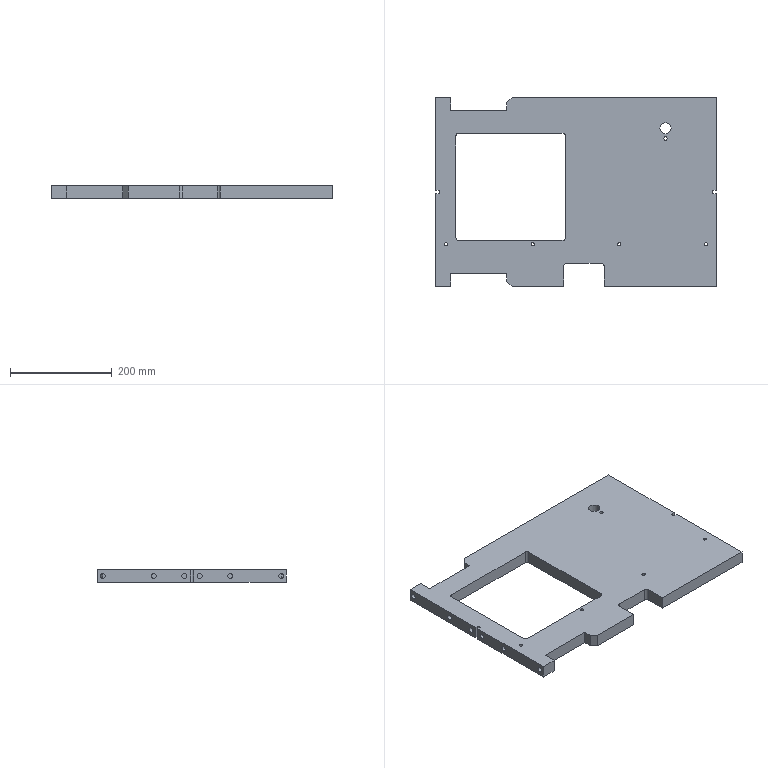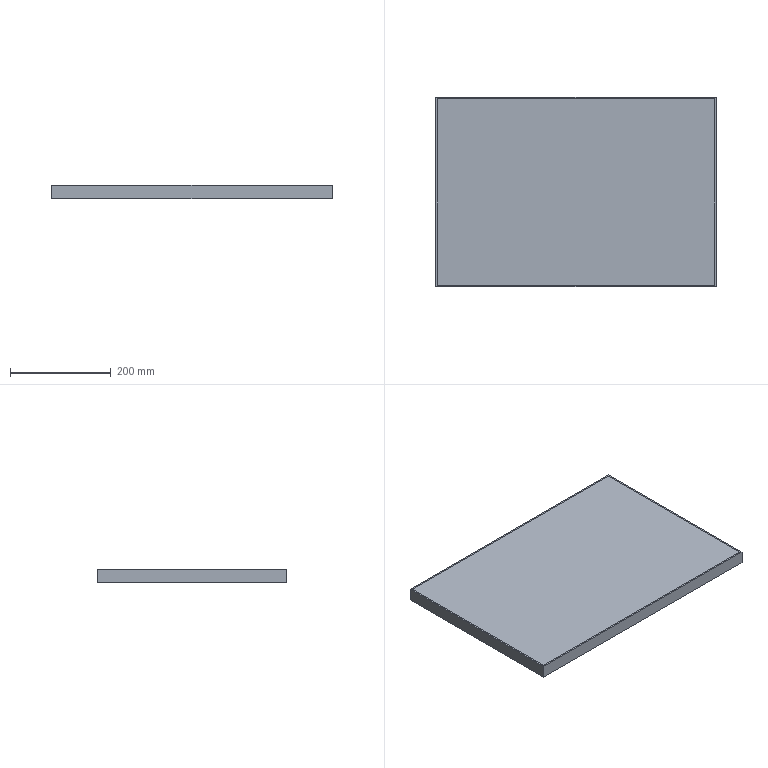CAM job | NX | 3-axis milling, drilling | part box 551 x 370 x 25 mm | stock box 557 x 376 x 26 mm
Tools:
number,name,description,diameter,corner_radius,flute_length,length,flutes
1,D50,Milling Tool-5 Parameters,50.0,0.0,50.0,75.0,2
2,D6A45,Milling Tool-5 Parameters,6.0,0.0,3.0,3.0,2
16,6.5ZT,Drilling Tool,6.5,0.0,35.0,50.0,2
3,D10,Milling Tool-5 Parameters,10.0,0.0,50.0,75.0,2
8,D6,Milling Tool-5 Parameters,6.0,0.0,50.0,75.0,2
10,D4,Milling Tool-5 Parameters,4.0,0.0,50.0,75.0,2
4,D10JING,Milling Tool-5 Parameters,10.0,0.0,50.0,75.0,2
Operations:
program,operation,operation_type,tool,method,geometry_group,spindle_rpm,surface_speed,feed_per_tooth,feed_cut,feed_plunge,cut_length_mm,path_length_mm,cut_time_min,machine_time_min
1-554-373-25毛胚-AB胶,FLOOR_WALL,VolumeBased25DMillingOperation,D50,METHOD,A,6500.0,1286.0,0.0962,1250.0,100.0,10079.997,10133.997,8.064,8.069
1-554-373-25毛胚-AB胶,DRILLING_COPY_1,Operation,D6A45,METHOD,A,3000.0,56.0,0.0333,200.0,0.0,27.6,882.732,0.138,0.2235
1-554-373-25毛胚-AB胶,DRILLING_COPY_1_COPY_COPY_1_COPY_1_COPY,Operation,6.5ZT,METHOD,A,2000.0,18.0,0.03,120.0,0.0,188.717,1204.965,1.573,1.674
1-554-373-25毛胚-AB胶,ZLEVEL_PROFILE,ZLevelMilling,D10,METHOD,A,7000.0,219.0,0.2143,3000.0,1000.0,51086.213,51167.613,17.06,17.068
1-554-373-25毛胚-AB胶,ZLEVEL_PROFILE_COPY,ZLevelMilling,D10,METHOD,A,7000.0,219.0,0.2143,3000.0,1000.0,21339.763,21920.462,7.177,7.235
1-554-373-25毛胚-AB胶,ZLEVEL_PROFILE_COPY_COPY_1_COPY_COPY_COPY_1_COPY_COPY_1,ZLevelMilling,D6,METHOD,A,7000.0,131.0,0.1071,1500.0,100.0,2070.238,4832.548,1.38,1.656
1-554-373-25毛胚-AB胶,ZLEVEL_PROFILE_COPY_COPY_1_COPY_COPY_COPY_1_COPY_COPY_1_COPY,ZLevelMilling,D4,METHOD,A,7000.0,65.0,0.0857,1200.0,100.0,1309.61,2829.834,1.091,1.243
1-554-373-25毛胚-AB胶,ZLEVEL_PROFILE_COPY_COPY_1_COPY_COPY_COPY_1_COPY_COPY_1_COPY_COPY,ZLevelMilling,D4,METHOD,A,7000.0,131.0,0.0857,1200.0,100.0,3082.296,4005.511,2.569,2.661
1-554-373-25毛胚-AB胶,ZLEVEL_PROFILE_COPY_1_1,ZLevelMilling,D10JING,METHOD,A,7000.0,219.0,0.0714,1000.0,1000.0,2495.004,2577.304,2.495,2.503
1-554-373-25毛胚-AB胶,ZLEVEL_PROFILE_COPY_COPY_1_COPY_COPY_COPY_1,ZLevelMilling,D10JING,METHOD,A,7000.0,219.0,0.0714,1000.0,100.0,82.632,192.878,0.0826,0.0937
1-554-373-25毛胚-AB胶,ZLEVEL_PROFILE_COPY_1_COPY_COPY_COPY_COPY_2_COPY,ZLevelMilling,D6A45,METHOD,A,7000.0,131.0,0.0714,1000.0,1000.0,3043.006,5584.979,3.043,3.297
1-554-373-25毛胚-AB胶,刀补13,ZLevelMilling,D4,METHOD,A,7000.0,131.0,0.0607,850.0,100.0,570.512,1367.457,0.6712,0.7509
1-554-373-25毛胚-AB胶,ZLEVEL_PROFILE_COPY_1_1_1,ZLevelMilling,D10JING,METHOD,A,7000.0,219.0,0.0714,1000.0,1000.0,8951.868,9035.618,8.952,8.96
2-554-373-25毛胚-AB胶,FLOOR_WALL_COPY,VolumeBased25DMillingOperation,D50,METHOD,B,6500.0,1286.0,0.0962,1250.0,100.0,9376.997,9430.997,7.502,7.507
2-554-373-25毛胚-AB胶,ZLEVEL_PROFILE_COPY_1_COPY_COPY_COPY_COPY_2_COPY_COPY,ZLevelMilling,D6A45,METHOD,B,7000.0,131.0,0.0714,1000.0,1000.0,3043.006,5784.137,3.043,3.317